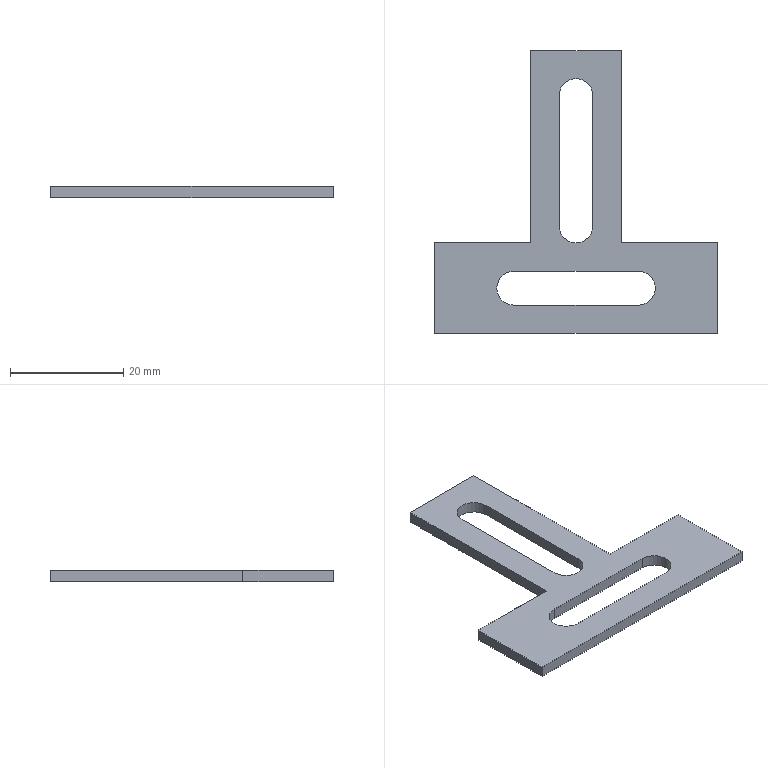Part | SolidWorks | features Extrusion 1 | 1 solid | 19 faces | box 50 x 50 x 2 mm | volume 2035 mm3 | plane 14 | cylinder 5 | commonest cylinder face diameters 6 x5
STEP:
#1=CARTESIAN_POINT('',(-11.,3.,2.));
#2=VERTEX_POINT('',#1);
#3=CARTESIAN_POINT('',(-14.,0.,2.));
#4=VERTEX_POINT('',#3);
#5=CARTESIAN_POINT('',(-11.,0.,2.));
#6=DIRECTION('',(0.,0.,1.));
#7=DIRECTION('',(1.,0.,0.));
#8=AXIS2_PLACEMENT_3D('',#5,#6,#7);
#9=CIRCLE('',#8,3.);
#10=EDGE_CURVE('',#2,#4,#9,.T.);
#11=ORIENTED_EDGE('',*,*,#10,.T.);
#12=CARTESIAN_POINT('',(-14.,0.,0.));
#13=VERTEX_POINT('',#12);
#14=CARTESIAN_POINT('',(-14.,0.,2.));
#15=DIRECTION('',(0.,0.,-1.));
#16=VECTOR('',#15,1000.);
#17=LINE('',#14,#16);
#18=EDGE_CURVE('',#4,#13,#17,.T.);
#19=ORIENTED_EDGE('',*,*,#18,.T.);
#20=CARTESIAN_POINT('',(-11.,3.,0.));
#21=VERTEX_POINT('',#20);
#22=CARTESIAN_POINT('',(-11.,0.,0.));
#23=DIRECTION('',(0.,0.,1.));
#24=DIRECTION('',(1.,0.,0.));
#25=AXIS2_PLACEMENT_3D('',#22,#23,#24);
#26=CIRCLE('',#25,3.);
#27=EDGE_CURVE('',#21,#13,#26,.T.);
#28=ORIENTED_EDGE('',*,*,#27,.F.);
#29=CARTESIAN_POINT('',(-11.,3.,2.));
#30=DIRECTION('',(0.,0.,-1.));
#31=VECTOR('',#30,1000.);
#32=LINE('',#29,#31);
#33=EDGE_CURVE('',#2,#21,#32,.T.);
#34=ORIENTED_EDGE('',*,*,#33,.F.);
#35=EDGE_LOOP('',(#11,#19,#28,#34));
#36=FACE_OUTER_BOUND('',#35,.T.);
#37=CARTESIAN_POINT('',(-11.,0.,2.));
#38=DIRECTION('',(0.,0.,-1.));
#39=DIRECTION('',(-1.,0.,0.));
#40=AXIS2_PLACEMENT_3D('',#37,#38,#39);
#41=CYLINDRICAL_SURFACE('',#40,3.);
#42=ADVANCED_FACE('',(#36),#41,.F.);
#43=CARTESIAN_POINT('',(-3.,11.,2.));
#44=VERTEX_POINT('',#43);
#45=CARTESIAN_POINT('',(3.,11.,2.));
#46=VERTEX_POINT('',#45);
#47=CARTESIAN_POINT('',(0.,11.,2.));
#48=DIRECTION('',(0.,0.,1.));
#49=DIRECTION('',(1.,0.,0.));
#50=AXIS2_PLACEMENT_3D('',#47,#48,#49);
#51=CIRCLE('',#50,3.);
#52=EDGE_CURVE('',#44,#46,#51,.T.);
#53=ORIENTED_EDGE('',*,*,#52,.F.);
#54=CARTESIAN_POINT('',(-3.,34.,2.));
#55=VERTEX_POINT('',#54);
#56=CARTESIAN_POINT('',(-3.,11.,2.));
#57=DIRECTION('',(0.,-1.,0.));
#58=VECTOR('',#57,1000.);
#59=LINE('',#56,#58);
#60=EDGE_CURVE('',#55,#44,#59,.T.);
#61=ORIENTED_EDGE('',*,*,#60,.F.);
#62=CARTESIAN_POINT('',(3.,34.,2.));
#63=VERTEX_POINT('',#62);
#64=CARTESIAN_POINT('',(0.,34.,2.));
#65=DIRECTION('',(0.,0.,1.));
#66=DIRECTION('',(1.,0.,0.));
#67=AXIS2_PLACEMENT_3D('',#64,#65,#66);
#68=CIRCLE('',#67,3.);
#69=EDGE_CURVE('',#63,#55,#68,.T.);
#70=ORIENTED_EDGE('',*,*,#69,.F.);
#71=CARTESIAN_POINT('',(3.,11.,2.));
#72=DIRECTION('',(0.,1.,0.));
#73=VECTOR('',#72,1000.);
#74=LINE('',#71,#73);
#75=EDGE_CURVE('',#46,#63,#74,.T.);
#76=ORIENTED_EDGE('',*,*,#75,.F.);
#77=EDGE_LOOP('',(#53,#61,#70,#76));
#78=FACE_BOUND('',#77,.T.);
#79=CARTESIAN_POINT('',(-8.,8.,2.));
#80=VERTEX_POINT('',#79);
#81=CARTESIAN_POINT('',(-25.,8.,2.));
#82=VERTEX_POINT('',#81);
#83=CARTESIAN_POINT('',(-8.,8.,2.));
#84=DIRECTION('',(-1.,0.,0.));
#85=VECTOR('',#84,1000.);
#86=LINE('',#83,#85);
#87=EDGE_CURVE('',#80,#82,#86,.T.);
#88=ORIENTED_EDGE('',*,*,#87,.T.);
#89=CARTESIAN_POINT('',(-25.,-8.,2.));
#90=VERTEX_POINT('',#89);
#91=CARTESIAN_POINT('',(-25.,-8.,2.));
#92=DIRECTION('',(0.,-1.,0.));
#93=VECTOR('',#92,1000.);
#94=LINE('',#91,#93);
#95=EDGE_CURVE('',#82,#90,#94,.T.);
#96=ORIENTED_EDGE('',*,*,#95,.T.);
#97=CARTESIAN_POINT('',(25.,-8.,2.));
#98=VERTEX_POINT('',#97);
#99=CARTESIAN_POINT('',(25.,-8.,2.));
#100=DIRECTION('',(1.,0.,0.));
#101=VECTOR('',#100,1000.);
#102=LINE('',#99,#101);
#103=EDGE_CURVE('',#90,#98,#102,.T.);
#104=ORIENTED_EDGE('',*,*,#103,.T.);
#105=CARTESIAN_POINT('',(25.,8.,2.));
#106=VERTEX_POINT('',#105);
#107=CARTESIAN_POINT('',(25.,-8.,2.));
#108=DIRECTION('',(0.,1.,0.));
#109=VECTOR('',#108,1000.);
#110=LINE('',#107,#109);
#111=EDGE_CURVE('',#98,#106,#110,.T.);
#112=ORIENTED_EDGE('',*,*,#111,.T.);
#113=CARTESIAN_POINT('',(8.,8.,2.));
#114=VERTEX_POINT('',#113);
#115=CARTESIAN_POINT('',(25.,8.,2.));
#116=DIRECTION('',(-1.,0.,0.));
#117=VECTOR('',#116,1000.);
#118=LINE('',#115,#117);
#119=EDGE_CURVE('',#106,#114,#118,.T.);
#120=ORIENTED_EDGE('',*,*,#119,.T.);
#121=CARTESIAN_POINT('',(8.,42.,2.));
#122=VERTEX_POINT('',#121);
#123=CARTESIAN_POINT('',(8.,42.,2.));
#124=DIRECTION('',(0.,1.,0.));
#125=VECTOR('',#124,1000.);
#126=LINE('',#123,#125);
#127=EDGE_CURVE('',#114,#122,#126,.T.);
#128=ORIENTED_EDGE('',*,*,#127,.T.);
#129=CARTESIAN_POINT('',(-8.,42.,2.));
#130=VERTEX_POINT('',#129);
#131=CARTESIAN_POINT('',(8.,42.,2.));
#132=DIRECTION('',(-1.,0.,0.));
#133=VECTOR('',#132,1000.);
#134=LINE('',#131,#133);
#135=EDGE_CURVE('',#122,#130,#134,.T.);
#136=ORIENTED_EDGE('',*,*,#135,.T.);
#137=CARTESIAN_POINT('',(-8.,42.,2.));
#138=DIRECTION('',(0.,-1.,0.));
#139=VECTOR('',#138,1000.);
#140=LINE('',#137,#139);
#141=EDGE_CURVE('',#130,#80,#140,.T.);
#142=ORIENTED_EDGE('',*,*,#141,.T.);
#143=EDGE_LOOP('',(#88,#96,#104,#112,#120,#128,#136,#142));
#144=FACE_OUTER_BOUND('',#143,.T.);
#145=ORIENTED_EDGE('',*,*,#10,.F.);
#146=CARTESIAN_POINT('',(11.,3.,2.));
#147=VERTEX_POINT('',#146);
#148=CARTESIAN_POINT('',(-11.,3.,2.));
#149=DIRECTION('',(-1.,0.,0.));
#150=VECTOR('',#149,1000.);
#151=LINE('',#148,#150);
#152=EDGE_CURVE('',#147,#2,#151,.T.);
#153=ORIENTED_EDGE('',*,*,#152,.F.);
#154=CARTESIAN_POINT('',(11.,-3.,2.));
#155=VERTEX_POINT('',#154);
#156=CARTESIAN_POINT('',(11.,0.,2.));
#157=DIRECTION('',(0.,0.,1.));
#158=DIRECTION('',(1.,0.,0.));
#159=AXIS2_PLACEMENT_3D('',#156,#157,#158);
#160=CIRCLE('',#159,3.);
#161=EDGE_CURVE('',#155,#147,#160,.T.);
#162=ORIENTED_EDGE('',*,*,#161,.F.);
#163=CARTESIAN_POINT('',(-11.,-3.,2.));
#164=VERTEX_POINT('',#163);
#165=CARTESIAN_POINT('',(-11.,-3.,2.));
#166=DIRECTION('',(1.,0.,0.));
#167=VECTOR('',#166,1000.);
#168=LINE('',#165,#167);
#169=EDGE_CURVE('',#164,#155,#168,.T.);
#170=ORIENTED_EDGE('',*,*,#169,.F.);
#171=CARTESIAN_POINT('',(-11.,0.,2.));
#172=DIRECTION('',(0.,0.,1.));
#173=DIRECTION('',(1.,0.,0.));
#174=AXIS2_PLACEMENT_3D('',#171,#172,#173);
#175=CIRCLE('',#174,3.);
#176=EDGE_CURVE('',#4,#164,#175,.T.);
#177=ORIENTED_EDGE('',*,*,#176,.F.);
#178=EDGE_LOOP('',(#145,#153,#162,#170,#177));
#179=FACE_BOUND('',#178,.T.);
#180=CARTESIAN_POINT('',(0.,0.,2.));
#181=DIRECTION('',(0.,0.,-1.));
#182=DIRECTION('',(-1.,0.,0.));
#183=AXIS2_PLACEMENT_3D('',#180,#181,#182);
#184=PLANE('',#183);
#185=ADVANCED_FACE('',(#78,#144,#179),#184,.F.);
#186=CARTESIAN_POINT('',(-8.,8.,0.));
#187=VERTEX_POINT('',#186);
#188=CARTESIAN_POINT('',(-25.,8.,0.));
#189=VERTEX_POINT('',#188);
#190=CARTESIAN_POINT('',(-8.,8.,0.));
#191=DIRECTION('',(-1.,0.,0.));
#192=VECTOR('',#191,1000.);
#193=LINE('',#190,#192);
#194=EDGE_CURVE('',#187,#189,#193,.T.);
#195=ORIENTED_EDGE('',*,*,#194,.F.);
#196=CARTESIAN_POINT('',(-8.,42.,0.));
#197=VERTEX_POINT('',#196);
#198=CARTESIAN_POINT('',(-8.,42.,0.));
#199=DIRECTION('',(0.,-1.,0.));
#200=VECTOR('',#199,1000.);
#201=LINE('',#198,#200);
#202=EDGE_CURVE('',#197,#187,#201,.T.);
#203=ORIENTED_EDGE('',*,*,#202,.F.);
#204=CARTESIAN_POINT('',(8.,42.,0.));
#205=VERTEX_POINT('',#204);
#206=CARTESIAN_POINT('',(8.,42.,0.));
#207=DIRECTION('',(-1.,0.,0.));
#208=VECTOR('',#207,1000.);
#209=LINE('',#206,#208);
#210=EDGE_CURVE('',#205,#197,#209,.T.);
#211=ORIENTED_EDGE('',*,*,#210,.F.);
#212=CARTESIAN_POINT('',(8.,8.,0.));
#213=VERTEX_POINT('',#212);
#214=CARTESIAN_POINT('',(8.,42.,0.));
#215=DIRECTION('',(0.,1.,0.));
#216=VECTOR('',#215,1000.);
#217=LINE('',#214,#216);
#218=EDGE_CURVE('',#213,#205,#217,.T.);
#219=ORIENTED_EDGE('',*,*,#218,.F.);
#220=CARTESIAN_POINT('',(25.,8.,0.));
#221=VERTEX_POINT('',#220);
#222=CARTESIAN_POINT('',(25.,8.,0.));
#223=DIRECTION('',(-1.,0.,0.));
#224=VECTOR('',#223,1000.);
#225=LINE('',#222,#224);
#226=EDGE_CURVE('',#221,#213,#225,.T.);
#227=ORIENTED_EDGE('',*,*,#226,.F.);
#228=CARTESIAN_POINT('',(25.,-8.,0.));
#229=VERTEX_POINT('',#228);
#230=CARTESIAN_POINT('',(25.,-8.,0.));
#231=DIRECTION('',(0.,1.,0.));
#232=VECTOR('',#231,1000.);
#233=LINE('',#230,#232);
#234=EDGE_CURVE('',#229,#221,#233,.T.);
#235=ORIENTED_EDGE('',*,*,#234,.F.);
#236=CARTESIAN_POINT('',(-25.,-8.,0.));
#237=VERTEX_POINT('',#236);
#238=CARTESIAN_POINT('',(25.,-8.,0.));
#239=DIRECTION('',(1.,0.,0.));
#240=VECTOR('',#239,1000.);
#241=LINE('',#238,#240);
#242=EDGE_CURVE('',#237,#229,#241,.T.);
#243=ORIENTED_EDGE('',*,*,#242,.F.);
#244=CARTESIAN_POINT('',(-25.,-8.,0.));
#245=DIRECTION('',(0.,-1.,0.));
#246=VECTOR('',#245,1000.);
#247=LINE('',#244,#246);
#248=EDGE_CURVE('',#189,#237,#247,.T.);
#249=ORIENTED_EDGE('',*,*,#248,.F.);
#250=EDGE_LOOP('',(#195,#203,#211,#219,#227,#235,#243,#249));
#251=FACE_OUTER_BOUND('',#250,.T.);
#252=CARTESIAN_POINT('',(-3.,34.,0.));
#253=VERTEX_POINT('',#252);
#254=CARTESIAN_POINT('',(-3.,11.,0.));
#255=VERTEX_POINT('',#254);
#256=CARTESIAN_POINT('',(-3.,11.,0.));
#257=DIRECTION('',(0.,-1.,0.));
#258=VECTOR('',#257,1000.);
#259=LINE('',#256,#258);
#260=EDGE_CURVE('',#253,#255,#259,.T.);
#261=ORIENTED_EDGE('',*,*,#260,.T.);
#262=CARTESIAN_POINT('',(3.,11.,0.));
#263=VERTEX_POINT('',#262);
#264=CARTESIAN_POINT('',(0.,11.,0.));
#265=DIRECTION('',(0.,0.,1.));
#266=DIRECTION('',(1.,0.,0.));
#267=AXIS2_PLACEMENT_3D('',#264,#265,#266);
#268=CIRCLE('',#267,3.);
#269=EDGE_CURVE('',#255,#263,#268,.T.);
#270=ORIENTED_EDGE('',*,*,#269,.T.);
#271=CARTESIAN_POINT('',(3.,34.,0.));
#272=VERTEX_POINT('',#271);
#273=CARTESIAN_POINT('',(3.,11.,0.));
#274=DIRECTION('',(0.,1.,0.));
#275=VECTOR('',#274,1000.);
#276=LINE('',#273,#275);
#277=EDGE_CURVE('',#263,#272,#276,.T.);
#278=ORIENTED_EDGE('',*,*,#277,.T.);
#279=CARTESIAN_POINT('',(0.,34.,0.));
#280=DIRECTION('',(0.,0.,1.));
#281=DIRECTION('',(1.,0.,0.));
#282=AXIS2_PLACEMENT_3D('',#279,#280,#281);
#283=CIRCLE('',#282,3.);
#284=EDGE_CURVE('',#272,#253,#283,.T.);
#285=ORIENTED_EDGE('',*,*,#284,.T.);
#286=EDGE_LOOP('',(#261,#270,#278,#285));
#287=FACE_BOUND('',#286,.T.);
#288=CARTESIAN_POINT('',(11.,3.,0.));
#289=VERTEX_POINT('',#288);
#290=CARTESIAN_POINT('',(-11.,3.,0.));
#291=DIRECTION('',(-1.,0.,0.));
#292=VECTOR('',#291,1000.);
#293=LINE('',#290,#292);
#294=EDGE_CURVE('',#289,#21,#293,.T.);
#295=ORIENTED_EDGE('',*,*,#294,.T.);
#296=ORIENTED_EDGE('',*,*,#27,.T.);
#297=CARTESIAN_POINT('',(-11.,-3.,0.));
#298=VERTEX_POINT('',#297);
#299=CARTESIAN_POINT('',(-11.,0.,0.));
#300=DIRECTION('',(0.,0.,1.));
#301=DIRECTION('',(1.,0.,0.));
#302=AXIS2_PLACEMENT_3D('',#299,#300,#301);
#303=CIRCLE('',#302,3.);
#304=EDGE_CURVE('',#13,#298,#303,.T.);
#305=ORIENTED_EDGE('',*,*,#304,.T.);
#306=CARTESIAN_POINT('',(11.,-3.,0.));
#307=VERTEX_POINT('',#306);
#308=CARTESIAN_POINT('',(-11.,-3.,0.));
#309=DIRECTION('',(1.,0.,0.));
#310=VECTOR('',#309,1000.);
#311=LINE('',#308,#310);
#312=EDGE_CURVE('',#298,#307,#311,.T.);
#313=ORIENTED_EDGE('',*,*,#312,.T.);
#314=CARTESIAN_POINT('',(11.,0.,0.));
#315=DIRECTION('',(0.,0.,1.));
#316=DIRECTION('',(1.,0.,0.));
#317=AXIS2_PLACEMENT_3D('',#314,#315,#316);
#318=CIRCLE('',#317,3.);
#319=EDGE_CURVE('',#307,#289,#318,.T.);
#320=ORIENTED_EDGE('',*,*,#319,.T.);
#321=EDGE_LOOP('',(#295,#296,#305,#313,#320));
#322=FACE_BOUND('',#321,.T.);
#323=CARTESIAN_POINT('',(0.,0.,0.));
#324=DIRECTION('',(0.,0.,-1.));
#325=DIRECTION('',(-1.,0.,0.));
#326=AXIS2_PLACEMENT_3D('',#323,#324,#325);
#327=PLANE('',#326);
#328=ADVANCED_FACE('',(#251,#287,#322),#327,.T.);
#329=ORIENTED_EDGE('',*,*,#194,.T.);
#330=CARTESIAN_POINT('',(-25.,8.,2.));
#331=DIRECTION('',(0.,0.,-1.));
#332=VECTOR('',#331,1000.);
#333=LINE('',#330,#332);
#334=EDGE_CURVE('',#82,#189,#333,.T.);
#335=ORIENTED_EDGE('',*,*,#334,.F.);
#336=ORIENTED_EDGE('',*,*,#87,.F.);
#337=CARTESIAN_POINT('',(-8.,8.,2.));
#338=DIRECTION('',(0.,0.,-1.));
#339=VECTOR('',#338,1000.);
#340=LINE('',#337,#339);
#341=EDGE_CURVE('',#80,#187,#340,.T.);
#342=ORIENTED_EDGE('',*,*,#341,.T.);
#343=EDGE_LOOP('',(#329,#335,#336,#342));
#344=FACE_OUTER_BOUND('',#343,.T.);
#345=CARTESIAN_POINT('',(-8.,8.,2.));
#346=DIRECTION('',(0.,-1.,0.));
#347=DIRECTION('',(1.,0.,0.));
#348=AXIS2_PLACEMENT_3D('',#345,#346,#347);
#349=PLANE('',#348);
#350=ADVANCED_FACE('',(#344),#349,.F.);
#351=ORIENTED_EDGE('',*,*,#248,.T.);
#352=CARTESIAN_POINT('',(-25.,-8.,2.));
#353=DIRECTION('',(0.,0.,-1.));
#354=VECTOR('',#353,1000.);
#355=LINE('',#352,#354);
#356=EDGE_CURVE('',#90,#237,#355,.T.);
#357=ORIENTED_EDGE('',*,*,#356,.F.);
#358=ORIENTED_EDGE('',*,*,#95,.F.);
#359=ORIENTED_EDGE('',*,*,#334,.T.);
#360=EDGE_LOOP('',(#351,#357,#358,#359));
#361=FACE_OUTER_BOUND('',#360,.T.);
#362=CARTESIAN_POINT('',(-25.,-8.,2.));
#363=DIRECTION('',(1.,0.,0.));
#364=DIRECTION('',(0.,0.,-1.));
#365=AXIS2_PLACEMENT_3D('',#362,#363,#364);
#366=PLANE('',#365);
#367=ADVANCED_FACE('',(#361),#366,.F.);
#368=ORIENTED_EDGE('',*,*,#242,.T.);
#369=CARTESIAN_POINT('',(25.,-8.,2.));
#370=DIRECTION('',(0.,0.,-1.));
#371=VECTOR('',#370,1000.);
#372=LINE('',#369,#371);
#373=EDGE_CURVE('',#98,#229,#372,.T.);
#374=ORIENTED_EDGE('',*,*,#373,.F.);
#375=ORIENTED_EDGE('',*,*,#103,.F.);
#376=ORIENTED_EDGE('',*,*,#356,.T.);
#377=EDGE_LOOP('',(#368,#374,#375,#376));
#378=FACE_OUTER_BOUND('',#377,.T.);
#379=CARTESIAN_POINT('',(25.,-8.,2.));
#380=DIRECTION('',(0.,1.,0.));
#381=DIRECTION('',(-1.,0.,0.));
#382=AXIS2_PLACEMENT_3D('',#379,#380,#381);
#383=PLANE('',#382);
#384=ADVANCED_FACE('',(#378),#383,.F.);
#385=ORIENTED_EDGE('',*,*,#234,.T.);
#386=CARTESIAN_POINT('',(25.,8.,2.));
#387=DIRECTION('',(0.,0.,-1.));
#388=VECTOR('',#387,1000.);
#389=LINE('',#386,#388);
#390=EDGE_CURVE('',#106,#221,#389,.T.);
#391=ORIENTED_EDGE('',*,*,#390,.F.);
#392=ORIENTED_EDGE('',*,*,#111,.F.);
#393=ORIENTED_EDGE('',*,*,#373,.T.);
#394=EDGE_LOOP('',(#385,#391,#392,#393));
#395=FACE_OUTER_BOUND('',#394,.T.);
#396=CARTESIAN_POINT('',(25.,-8.,2.));
#397=DIRECTION('',(-1.,0.,0.));
#398=DIRECTION('',(0.,0.,1.));
#399=AXIS2_PLACEMENT_3D('',#396,#397,#398);
#400=PLANE('',#399);
#401=ADVANCED_FACE('',(#395),#400,.F.);
#402=ORIENTED_EDGE('',*,*,#226,.T.);
#403=CARTESIAN_POINT('',(8.,8.,2.));
#404=DIRECTION('',(0.,0.,-1.));
#405=VECTOR('',#404,1000.);
#406=LINE('',#403,#405);
#407=EDGE_CURVE('',#114,#213,#406,.T.);
#408=ORIENTED_EDGE('',*,*,#407,.F.);
#409=ORIENTED_EDGE('',*,*,#119,.F.);
#410=ORIENTED_EDGE('',*,*,#390,.T.);
#411=EDGE_LOOP('',(#402,#408,#409,#410));
#412=FACE_OUTER_BOUND('',#411,.T.);
#413=CARTESIAN_POINT('',(25.,8.,2.));
#414=DIRECTION('',(0.,-1.,0.));
#415=DIRECTION('',(1.,0.,0.));
#416=AXIS2_PLACEMENT_3D('',#413,#414,#415);
#417=PLANE('',#416);
#418=ADVANCED_FACE('',(#412),#417,.F.);
#419=ORIENTED_EDGE('',*,*,#218,.T.);
#420=CARTESIAN_POINT('',(8.,42.,2.));
#421=DIRECTION('',(0.,0.,-1.));
#422=VECTOR('',#421,1000.);
#423=LINE('',#420,#422);
#424=EDGE_CURVE('',#122,#205,#423,.T.);
#425=ORIENTED_EDGE('',*,*,#424,.F.);
#426=ORIENTED_EDGE('',*,*,#127,.F.);
#427=ORIENTED_EDGE('',*,*,#407,.T.);
#428=EDGE_LOOP('',(#419,#425,#426,#427));
#429=FACE_OUTER_BOUND('',#428,.T.);
#430=CARTESIAN_POINT('',(8.,42.,2.));
#431=DIRECTION('',(-1.,0.,0.));
#432=DIRECTION('',(0.,-1.,0.));
#433=AXIS2_PLACEMENT_3D('',#430,#431,#432);
#434=PLANE('',#433);
#435=ADVANCED_FACE('',(#429),#434,.F.);
#436=ORIENTED_EDGE('',*,*,#210,.T.);
#437=CARTESIAN_POINT('',(-8.,42.,2.));
#438=DIRECTION('',(0.,0.,-1.));
#439=VECTOR('',#438,1000.);
#440=LINE('',#437,#439);
#441=EDGE_CURVE('',#130,#197,#440,.T.);
#442=ORIENTED_EDGE('',*,*,#441,.F.);
#443=ORIENTED_EDGE('',*,*,#135,.F.);
#444=ORIENTED_EDGE('',*,*,#424,.T.);
#445=EDGE_LOOP('',(#436,#442,#443,#444));
#446=FACE_OUTER_BOUND('',#445,.T.);
#447=CARTESIAN_POINT('',(8.,42.,2.));
#448=DIRECTION('',(0.,-1.,0.));
#449=DIRECTION('',(0.,0.,-1.));
#450=AXIS2_PLACEMENT_3D('',#447,#448,#449);
#451=PLANE('',#450);
#452=ADVANCED_FACE('',(#446),#451,.F.);
#453=ORIENTED_EDGE('',*,*,#202,.T.);
#454=ORIENTED_EDGE('',*,*,#341,.F.);
#455=ORIENTED_EDGE('',*,*,#141,.F.);
#456=ORIENTED_EDGE('',*,*,#441,.T.);
#457=EDGE_LOOP('',(#453,#454,#455,#456));
#458=FACE_OUTER_BOUND('',#457,.T.);
#459=CARTESIAN_POINT('',(-8.,42.,2.));
#460=DIRECTION('',(1.,0.,0.));
#461=DIRECTION('',(0.,1.,0.));
#462=AXIS2_PLACEMENT_3D('',#459,#460,#461);
#463=PLANE('',#462);
#464=ADVANCED_FACE('',(#458),#463,.F.);
#465=ORIENTED_EDGE('',*,*,#269,.F.);
#466=CARTESIAN_POINT('',(-3.,11.,2.));
#467=DIRECTION('',(0.,0.,-1.));
#468=VECTOR('',#467,1000.);
#469=LINE('',#466,#468);
#470=EDGE_CURVE('',#44,#255,#469,.T.);
#471=ORIENTED_EDGE('',*,*,#470,.F.);
#472=ORIENTED_EDGE('',*,*,#52,.T.);
#473=CARTESIAN_POINT('',(3.,11.,2.));
#474=DIRECTION('',(0.,0.,-1.));
#475=VECTOR('',#474,1000.);
#476=LINE('',#473,#475);
#477=EDGE_CURVE('',#46,#263,#476,.T.);
#478=ORIENTED_EDGE('',*,*,#477,.T.);
#479=EDGE_LOOP('',(#465,#471,#472,#478));
#480=FACE_OUTER_BOUND('',#479,.T.);
#481=CARTESIAN_POINT('',(0.,11.,2.));
#482=DIRECTION('',(0.,0.,-1.));
#483=DIRECTION('',(-1.,0.,0.));
#484=AXIS2_PLACEMENT_3D('',#481,#482,#483);
#485=CYLINDRICAL_SURFACE('',#484,3.);
#486=ADVANCED_FACE('',(#480),#485,.F.);
#487=ORIENTED_EDGE('',*,*,#277,.F.);
#488=ORIENTED_EDGE('',*,*,#477,.F.);
#489=ORIENTED_EDGE('',*,*,#75,.T.);
#490=CARTESIAN_POINT('',(3.,34.,2.));
#491=DIRECTION('',(0.,0.,-1.));
#492=VECTOR('',#491,1000.);
#493=LINE('',#490,#492);
#494=EDGE_CURVE('',#63,#272,#493,.T.);
#495=ORIENTED_EDGE('',*,*,#494,.T.);
#496=EDGE_LOOP('',(#487,#488,#489,#495));
#497=FACE_OUTER_BOUND('',#496,.T.);
#498=CARTESIAN_POINT('',(3.,11.,2.));
#499=DIRECTION('',(-1.,0.,0.));
#500=DIRECTION('',(0.,0.,1.));
#501=AXIS2_PLACEMENT_3D('',#498,#499,#500);
#502=PLANE('',#501);
#503=ADVANCED_FACE('',(#497),#502,.T.);
#504=ORIENTED_EDGE('',*,*,#284,.F.);
#505=ORIENTED_EDGE('',*,*,#494,.F.);
#506=ORIENTED_EDGE('',*,*,#69,.T.);
#507=CARTESIAN_POINT('',(-3.,34.,2.));
#508=DIRECTION('',(0.,0.,-1.));
#509=VECTOR('',#508,1000.);
#510=LINE('',#507,#509);
#511=EDGE_CURVE('',#55,#253,#510,.T.);
#512=ORIENTED_EDGE('',*,*,#511,.T.);
#513=EDGE_LOOP('',(#504,#505,#506,#512));
#514=FACE_OUTER_BOUND('',#513,.T.);
#515=CARTESIAN_POINT('',(0.,34.,2.));
#516=DIRECTION('',(0.,0.,-1.));
#517=DIRECTION('',(-1.,0.,0.));
#518=AXIS2_PLACEMENT_3D('',#515,#516,#517);
#519=CYLINDRICAL_SURFACE('',#518,3.);
#520=ADVANCED_FACE('',(#514),#519,.F.);
#521=ORIENTED_EDGE('',*,*,#260,.F.);
#522=ORIENTED_EDGE('',*,*,#511,.F.);
#523=ORIENTED_EDGE('',*,*,#60,.T.);
#524=ORIENTED_EDGE('',*,*,#470,.T.);
#525=EDGE_LOOP('',(#521,#522,#523,#524));
#526=FACE_OUTER_BOUND('',#525,.T.);
#527=CARTESIAN_POINT('',(-3.,11.,2.));
#528=DIRECTION('',(1.,0.,0.));
#529=DIRECTION('',(0.,0.,-1.));
#530=AXIS2_PLACEMENT_3D('',#527,#528,#529);
#531=PLANE('',#530);
#532=ADVANCED_FACE('',(#526),#531,.T.);
#533=ORIENTED_EDGE('',*,*,#18,.F.);
#534=ORIENTED_EDGE('',*,*,#176,.T.);
#535=CARTESIAN_POINT('',(-11.,-3.,2.));
#536=DIRECTION('',(0.,0.,-1.));
#537=VECTOR('',#536,1000.);
#538=LINE('',#535,#537);
#539=EDGE_CURVE('',#164,#298,#538,.T.);
#540=ORIENTED_EDGE('',*,*,#539,.T.);
#541=ORIENTED_EDGE('',*,*,#304,.F.);
#542=EDGE_LOOP('',(#533,#534,#540,#541));
#543=FACE_OUTER_BOUND('',#542,.T.);
#544=CARTESIAN_POINT('',(-11.,0.,2.));
#545=DIRECTION('',(0.,0.,-1.));
#546=DIRECTION('',(-1.,0.,0.));
#547=AXIS2_PLACEMENT_3D('',#544,#545,#546);
#548=CYLINDRICAL_SURFACE('',#547,3.);
#549=ADVANCED_FACE('',(#543),#548,.F.);
#550=ORIENTED_EDGE('',*,*,#312,.F.);
#551=ORIENTED_EDGE('',*,*,#539,.F.);
#552=ORIENTED_EDGE('',*,*,#169,.T.);
#553=CARTESIAN_POINT('',(11.,-3.,2.));
#554=DIRECTION('',(0.,0.,-1.));
#555=VECTOR('',#554,1000.);
#556=LINE('',#553,#555);
#557=EDGE_CURVE('',#155,#307,#556,.T.);
#558=ORIENTED_EDGE('',*,*,#557,.T.);
#559=EDGE_LOOP('',(#550,#551,#552,#558));
#560=FACE_OUTER_BOUND('',#559,.T.);
#561=CARTESIAN_POINT('',(-11.,-3.,2.));
#562=DIRECTION('',(0.,1.,0.));
#563=DIRECTION('',(-1.,0.,0.));
#564=AXIS2_PLACEMENT_3D('',#561,#562,#563);
#565=PLANE('',#564);
#566=ADVANCED_FACE('',(#560),#565,.T.);
#567=ORIENTED_EDGE('',*,*,#319,.F.);
#568=ORIENTED_EDGE('',*,*,#557,.F.);
#569=ORIENTED_EDGE('',*,*,#161,.T.);
#570=CARTESIAN_POINT('',(11.,3.,2.));
#571=DIRECTION('',(0.,0.,-1.));
#572=VECTOR('',#571,1000.);
#573=LINE('',#570,#572);
#574=EDGE_CURVE('',#147,#289,#573,.T.);
#575=ORIENTED_EDGE('',*,*,#574,.T.);
#576=EDGE_LOOP('',(#567,#568,#569,#575));
#577=FACE_OUTER_BOUND('',#576,.T.);
#578=CARTESIAN_POINT('',(11.,0.,2.));
#579=DIRECTION('',(0.,0.,-1.));
#580=DIRECTION('',(-1.,0.,0.));
#581=AXIS2_PLACEMENT_3D('',#578,#579,#580);
#582=CYLINDRICAL_SURFACE('',#581,3.);
#583=ADVANCED_FACE('',(#577),#582,.F.);
#584=ORIENTED_EDGE('',*,*,#294,.F.);
#585=ORIENTED_EDGE('',*,*,#574,.F.);
#586=ORIENTED_EDGE('',*,*,#152,.T.);
#587=ORIENTED_EDGE('',*,*,#33,.T.);
#588=EDGE_LOOP('',(#584,#585,#586,#587));
#589=FACE_OUTER_BOUND('',#588,.T.);
#590=CARTESIAN_POINT('',(-11.,3.,2.));
#591=DIRECTION('',(0.,-1.,0.));
#592=DIRECTION('',(0.,0.,-1.));
#593=AXIS2_PLACEMENT_3D('',#590,#591,#592);
#594=PLANE('',#593);
#595=ADVANCED_FACE('',(#589),#594,.T.);
#596=CLOSED_SHELL('',(#42,#185,#328,#350,#367,#384,#401,#418,#435,#452,#464,#486,#503,#520,#532,#549,#566,#583,#595));
#597=MANIFOLD_SOLID_BREP('',#596);
#598=CARTESIAN_POINT('',(0.,0.,0.));
#599=DIRECTION('',(0.,0.,1.));
#600=DIRECTION('',(1.,0.,0.));
#601=AXIS2_PLACEMENT_3D('',#598,#599,#600);
#602=(LENGTH_UNIT()NAMED_UNIT(*)SI_UNIT(.MILLI.,.METRE.));
#603=UNCERTAINTY_MEASURE_WITH_UNIT(LENGTH_MEASURE(0.00001),#602,'','');
#604=(NAMED_UNIT(*)PLANE_ANGLE_UNIT()SI_UNIT($,.RADIAN.));
#605=(NAMED_UNIT(*)SI_UNIT($,.STERADIAN.)SOLID_ANGLE_UNIT());
#606=(GEOMETRIC_REPRESENTATION_CONTEXT(3)GLOBAL_UNCERTAINTY_ASSIGNED_CONTEXT((#603))GLOBAL_UNIT_ASSIGNED_CONTEXT((#602,#604,#605))REPRESENTATION_CONTEXT('',''));
#607=ADVANCED_BREP_SHAPE_REPRESENTATION('',(#597,#601),#606);